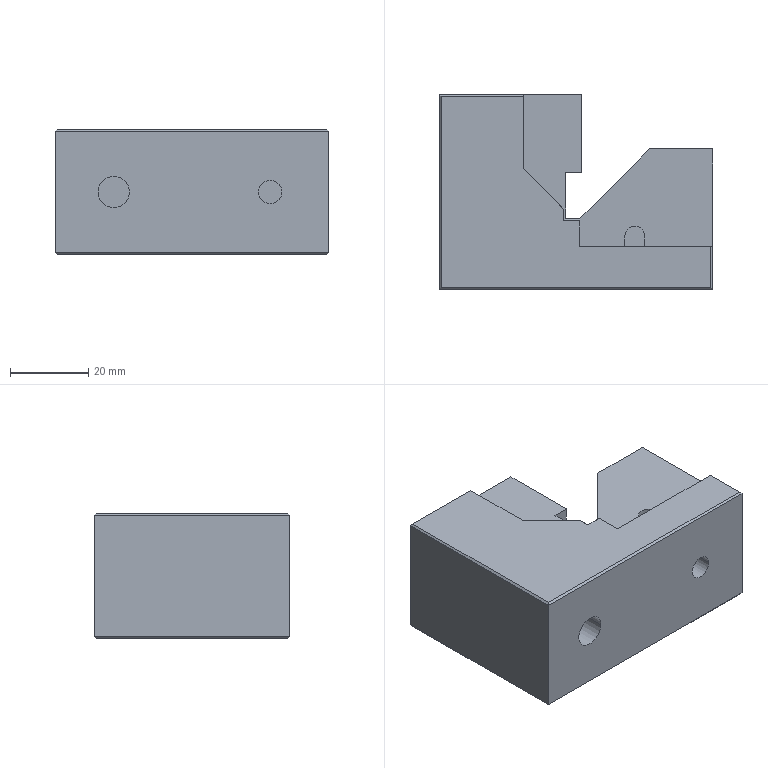Part | STEP file | product fixture | 1 solid | 50 faces | box 70 x 50 x 32 mm | volume 81575 mm3 | plane 44 | cylinder 6 | commonest cylinder face diameters 5 x2 6 x2 8 x2